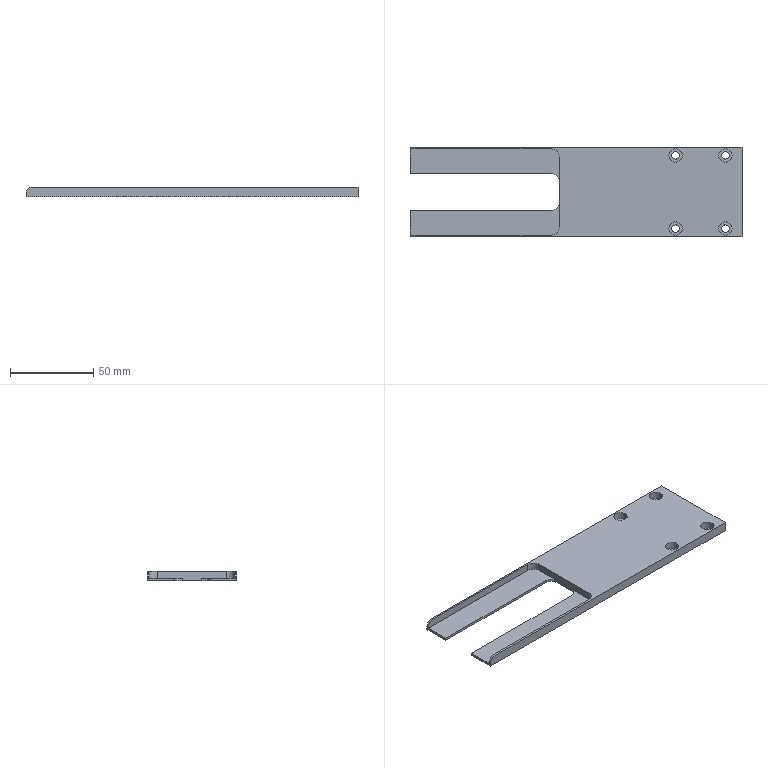Part | STEP file | PN_0092 Mount electronic clip plate | 1 solid | 40 faces | box 200 x 54 x 6 mm | volume 39814 mm3 | cylinder 22 | plane 18 | commonest cylinder face diameters 8 x10 4.5 x8 10 x4